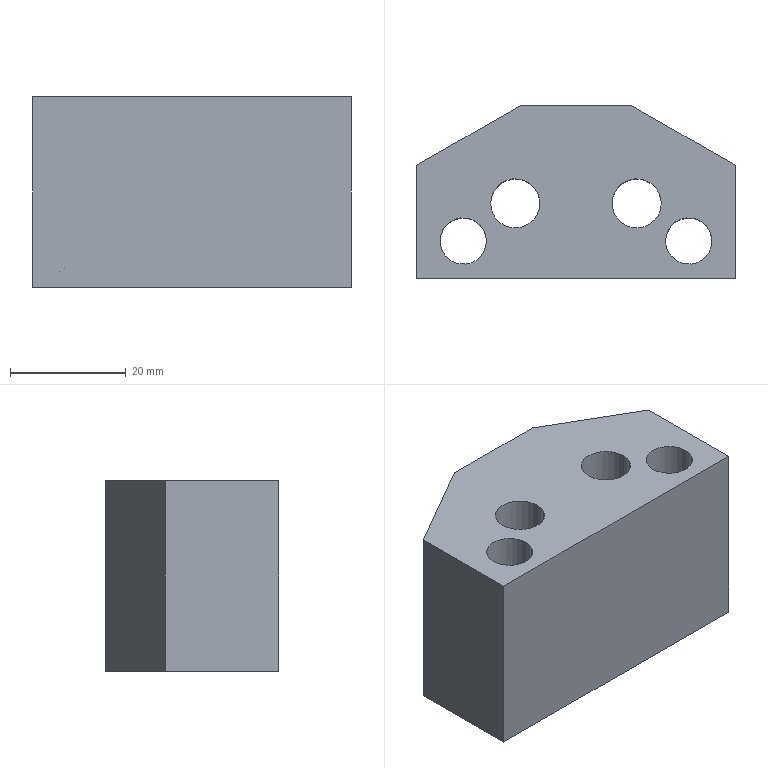Part | CATIA | 1 solid | 16 faces | box 55 x 30 x 33 mm | volume 41214 mm3 | plane 8 | cylinder 8 | commonest cylinder face diameters 8 x4 8.5 x4
STEP:
#1=CARTESIAN_POINT('',(27.5,-30.,38.));
#2=VERTEX_POINT('',#1);
#3=CARTESIAN_POINT('',(27.5,-30.,5.));
#4=VERTEX_POINT('',#3);
#5=CARTESIAN_POINT('',(27.5,-30.,21.5));
#6=DIRECTION('',(0.,0.,-1.));
#7=VECTOR('',#6,1.);
#8=LINE('',#5,#7);
#9=EDGE_CURVE('',#2,#4,#8,.T.);
#10=ORIENTED_EDGE('',*,*,#9,.F.);
#11=CARTESIAN_POINT('',(-27.5,-30.,38.));
#12=VERTEX_POINT('',#11);
#13=CARTESIAN_POINT('',(0.,-30.,38.));
#14=DIRECTION('',(-1.,0.,0.));
#15=VECTOR('',#14,1.);
#16=LINE('',#13,#15);
#17=EDGE_CURVE('',#2,#12,#16,.T.);
#18=ORIENTED_EDGE('',*,*,#17,.T.);
#19=CARTESIAN_POINT('',(-27.5,-30.,5.));
#20=VERTEX_POINT('',#19);
#21=CARTESIAN_POINT('',(-27.5,-30.,21.5));
#22=DIRECTION('',(0.,0.,-1.));
#23=VECTOR('',#22,1.);
#24=LINE('',#21,#23);
#25=EDGE_CURVE('',#12,#20,#24,.T.);
#26=ORIENTED_EDGE('',*,*,#25,.T.);
#27=CARTESIAN_POINT('',(0.,-30.,5.));
#28=DIRECTION('',(-1.,0.,0.));
#29=VECTOR('',#28,1.);
#30=LINE('',#27,#29);
#31=EDGE_CURVE('',#4,#20,#30,.T.);
#32=ORIENTED_EDGE('',*,*,#31,.F.);
#33=EDGE_LOOP('',(#10,#18,#26,#32));
#34=FACE_OUTER_BOUND('',#33,.T.);
#35=CARTESIAN_POINT('',(27.5,-30.,38.));
#36=DIRECTION('',(0.,-1.,0.));
#37=DIRECTION('',(-1.,0.,0.));
#38=AXIS2_PLACEMENT_3D('',#35,#36,#37);
#39=PLANE('',#38);
#40=ADVANCED_FACE('',(#34),#39,.T.);
#41=CARTESIAN_POINT('',(-27.5,-10.392,38.));
#42=VERTEX_POINT('',#41);
#43=CARTESIAN_POINT('',(-27.5,-10.392,5.));
#44=VERTEX_POINT('',#43);
#45=CARTESIAN_POINT('',(-27.5,-10.392,21.5));
#46=DIRECTION('',(0.,0.,-1.));
#47=VECTOR('',#46,1.);
#48=LINE('',#45,#47);
#49=EDGE_CURVE('',#42,#44,#48,.T.);
#50=ORIENTED_EDGE('',*,*,#49,.T.);
#51=CARTESIAN_POINT('',(-27.5,-20.196,5.));
#52=DIRECTION('',(0.,-1.,0.));
#53=VECTOR('',#52,1.);
#54=LINE('',#51,#53);
#55=EDGE_CURVE('',#20,#44,#54,.F.);
#56=ORIENTED_EDGE('',*,*,#55,.F.);
#57=ORIENTED_EDGE('',*,*,#25,.F.);
#58=CARTESIAN_POINT('',(-27.5,-20.196,38.));
#59=DIRECTION('',(0.,-1.,0.));
#60=VECTOR('',#59,1.);
#61=LINE('',#58,#60);
#62=EDGE_CURVE('',#12,#42,#61,.F.);
#63=ORIENTED_EDGE('',*,*,#62,.T.);
#64=EDGE_LOOP('',(#50,#56,#57,#63));
#65=FACE_OUTER_BOUND('',#64,.T.);
#66=CARTESIAN_POINT('',(-27.5,0.,38.));
#67=DIRECTION('',(1.,0.,0.));
#68=DIRECTION('',(0.,-1.,0.));
#69=AXIS2_PLACEMENT_3D('',#66,#67,#68);
#70=PLANE('',#69);
#71=ADVANCED_FACE('',(#65),#70,.F.);
#72=CARTESIAN_POINT('',(-9.5,0.,5.));
#73=VERTEX_POINT('',#72);
#74=CARTESIAN_POINT('',(-18.5,-5.196,5.));
#75=DIRECTION('',(-0.866,-0.5,0.));
#76=VECTOR('',#75,1.);
#77=LINE('',#74,#76);
#78=EDGE_CURVE('',#73,#44,#77,.T.);
#79=ORIENTED_EDGE('',*,*,#78,.T.);
#80=ORIENTED_EDGE('',*,*,#49,.F.);
#81=CARTESIAN_POINT('',(-9.5,0.,38.));
#82=VERTEX_POINT('',#81);
#83=CARTESIAN_POINT('',(-18.5,-5.196,38.));
#84=DIRECTION('',(-0.866,-0.5,0.));
#85=VECTOR('',#84,1.);
#86=LINE('',#83,#85);
#87=EDGE_CURVE('',#42,#82,#86,.F.);
#88=ORIENTED_EDGE('',*,*,#87,.T.);
#89=CARTESIAN_POINT('',(-9.5,0.,21.5));
#90=DIRECTION('',(0.,0.,-1.));
#91=VECTOR('',#90,1.);
#92=LINE('',#89,#91);
#93=EDGE_CURVE('',#82,#73,#92,.T.);
#94=ORIENTED_EDGE('',*,*,#93,.T.);
#95=EDGE_LOOP('',(#79,#80,#88,#94));
#96=FACE_OUTER_BOUND('',#95,.T.);
#97=CARTESIAN_POINT('',(-9.5,0.,44.6));
#98=DIRECTION('',(-0.5,0.866,0.));
#99=DIRECTION('',(0.,0.,-1.));
#100=AXIS2_PLACEMENT_3D('',#97,#98,#99);
#101=PLANE('',#100);
#102=ADVANCED_FACE('',(#96),#101,.T.);
#103=CARTESIAN_POINT('',(27.5,-10.392,38.));
#104=VERTEX_POINT('',#103);
#105=CARTESIAN_POINT('',(27.5,-10.392,5.));
#106=VERTEX_POINT('',#105);
#107=CARTESIAN_POINT('',(27.5,-10.392,21.5));
#108=DIRECTION('',(0.,0.,1.));
#109=VECTOR('',#108,1.);
#110=LINE('',#107,#109);
#111=EDGE_CURVE('',#104,#106,#110,.F.);
#112=ORIENTED_EDGE('',*,*,#111,.F.);
#113=CARTESIAN_POINT('',(27.5,-20.196,38.));
#114=DIRECTION('',(0.,1.,0.));
#115=VECTOR('',#114,1.);
#116=LINE('',#113,#115);
#117=EDGE_CURVE('',#104,#2,#116,.F.);
#118=ORIENTED_EDGE('',*,*,#117,.T.);
#119=ORIENTED_EDGE('',*,*,#9,.T.);
#120=CARTESIAN_POINT('',(27.5,-20.196,5.));
#121=DIRECTION('',(0.,1.,0.));
#122=VECTOR('',#121,1.);
#123=LINE('',#120,#122);
#124=EDGE_CURVE('',#106,#4,#123,.F.);
#125=ORIENTED_EDGE('',*,*,#124,.F.);
#126=EDGE_LOOP('',(#112,#118,#119,#125));
#127=FACE_OUTER_BOUND('',#126,.T.);
#128=CARTESIAN_POINT('',(27.5,-30.,38.));
#129=DIRECTION('',(-1.,0.,0.));
#130=DIRECTION('',(0.,1.,0.));
#131=AXIS2_PLACEMENT_3D('',#128,#129,#130);
#132=PLANE('',#131);
#133=ADVANCED_FACE('',(#127),#132,.F.);
#134=CARTESIAN_POINT('',(9.5,0.,5.));
#135=VERTEX_POINT('',#134);
#136=CARTESIAN_POINT('',(0.,0.,5.));
#137=DIRECTION('',(1.,0.,0.));
#138=VECTOR('',#137,1.);
#139=LINE('',#136,#138);
#140=EDGE_CURVE('',#73,#135,#139,.T.);
#141=ORIENTED_EDGE('',*,*,#140,.F.);
#142=ORIENTED_EDGE('',*,*,#93,.F.);
#143=CARTESIAN_POINT('',(9.5,0.,38.));
#144=VERTEX_POINT('',#143);
#145=CARTESIAN_POINT('',(0.,0.,38.));
#146=DIRECTION('',(1.,0.,0.));
#147=VECTOR('',#146,1.);
#148=LINE('',#145,#147);
#149=EDGE_CURVE('',#82,#144,#148,.T.);
#150=ORIENTED_EDGE('',*,*,#149,.T.);
#151=CARTESIAN_POINT('',(9.5,0.,21.5));
#152=DIRECTION('',(0.,0.,1.));
#153=VECTOR('',#152,1.);
#154=LINE('',#151,#153);
#155=EDGE_CURVE('',#144,#135,#154,.F.);
#156=ORIENTED_EDGE('',*,*,#155,.T.);
#157=EDGE_LOOP('',(#141,#142,#150,#156));
#158=FACE_OUTER_BOUND('',#157,.T.);
#159=CARTESIAN_POINT('',(-27.5,0.,38.));
#160=DIRECTION('',(0.,1.,0.));
#161=DIRECTION('',(1.,0.,0.));
#162=AXIS2_PLACEMENT_3D('',#159,#160,#161);
#163=PLANE('',#162);
#164=ADVANCED_FACE('',(#158),#163,.T.);
#165=CARTESIAN_POINT('',(18.5,-5.196,5.));
#166=DIRECTION('',(0.866,-0.5,0.));
#167=VECTOR('',#166,1.);
#168=LINE('',#165,#167);
#169=EDGE_CURVE('',#106,#135,#168,.F.);
#170=ORIENTED_EDGE('',*,*,#169,.T.);
#171=ORIENTED_EDGE('',*,*,#155,.F.);
#172=CARTESIAN_POINT('',(18.5,-5.196,38.));
#173=DIRECTION('',(0.866,-0.5,0.));
#174=VECTOR('',#173,1.);
#175=LINE('',#172,#174);
#176=EDGE_CURVE('',#144,#104,#175,.T.);
#177=ORIENTED_EDGE('',*,*,#176,.T.);
#178=ORIENTED_EDGE('',*,*,#111,.T.);
#179=EDGE_LOOP('',(#170,#171,#177,#178));
#180=FACE_OUTER_BOUND('',#179,.T.);
#181=CARTESIAN_POINT('',(9.5,0.,-1.6));
#182=DIRECTION('',(0.5,0.866,0.));
#183=DIRECTION('',(0.,0.,1.));
#184=AXIS2_PLACEMENT_3D('',#181,#182,#183);
#185=PLANE('',#184);
#186=ADVANCED_FACE('',(#180),#185,.T.);
#187=ORIENTED_EDGE('',*,*,#124,.T.);
#188=ORIENTED_EDGE('',*,*,#31,.T.);
#189=ORIENTED_EDGE('',*,*,#55,.T.);
#190=ORIENTED_EDGE('',*,*,#78,.F.);
#191=ORIENTED_EDGE('',*,*,#140,.T.);
#192=ORIENTED_EDGE('',*,*,#169,.F.);
#193=EDGE_LOOP('',(#187,#188,#189,#190,#191,#192));
#194=FACE_OUTER_BOUND('',#193,.T.);
#195=CARTESIAN_POINT('',(-14.23,-14.962,5.));
#196=VERTEX_POINT('',#195);
#197=CARTESIAN_POINT('',(-6.77,-19.038,5.));
#198=VERTEX_POINT('',#197);
#199=CARTESIAN_POINT('',(-10.5,-17.,5.));
#200=DIRECTION('',(0.,0.,-1.));
#201=AXIS2_PLACEMENT_3D('',#199,#200,$);
#202=CIRCLE('',#201,4.25);
#203=EDGE_CURVE('',#196,#198,#202,.T.);
#204=ORIENTED_EDGE('',*,*,#203,.F.);
#205=CARTESIAN_POINT('',(-10.5,-17.,5.));
#206=DIRECTION('',(0.,0.,-1.));
#207=AXIS2_PLACEMENT_3D('',#205,#206,$);
#208=CIRCLE('',#207,4.25);
#209=EDGE_CURVE('',#198,#196,#208,.T.);
#210=ORIENTED_EDGE('',*,*,#209,.F.);
#211=EDGE_LOOP('',(#204,#210));
#212=FACE_BOUND('',#211,.T.);
#213=CARTESIAN_POINT('',(6.77,-14.962,5.));
#214=VERTEX_POINT('',#213);
#215=CARTESIAN_POINT('',(14.23,-19.038,5.));
#216=VERTEX_POINT('',#215);
#217=CARTESIAN_POINT('',(10.5,-17.,5.));
#218=DIRECTION('',(0.,0.,-1.));
#219=AXIS2_PLACEMENT_3D('',#217,#218,$);
#220=CIRCLE('',#219,4.25);
#221=EDGE_CURVE('',#214,#216,#220,.T.);
#222=ORIENTED_EDGE('',*,*,#221,.F.);
#223=CARTESIAN_POINT('',(10.5,-17.,5.));
#224=DIRECTION('',(0.,0.,-1.));
#225=AXIS2_PLACEMENT_3D('',#223,#224,$);
#226=CIRCLE('',#225,4.25);
#227=EDGE_CURVE('',#216,#214,#226,.T.);
#228=ORIENTED_EDGE('',*,*,#227,.F.);
#229=EDGE_LOOP('',(#222,#228));
#230=FACE_BOUND('',#229,.T.);
#231=CARTESIAN_POINT('',(-23.01,-21.582,5.));
#232=VERTEX_POINT('',#231);
#233=CARTESIAN_POINT('',(-15.99,-25.418,5.));
#234=VERTEX_POINT('',#233);
#235=CARTESIAN_POINT('',(-19.5,-23.5,5.));
#236=DIRECTION('',(0.,0.,-1.));
#237=AXIS2_PLACEMENT_3D('',#235,#236,$);
#238=CIRCLE('',#237,4.);
#239=EDGE_CURVE('',#232,#234,#238,.T.);
#240=ORIENTED_EDGE('',*,*,#239,.F.);
#241=CARTESIAN_POINT('',(-19.5,-23.5,5.));
#242=DIRECTION('',(0.,0.,-1.));
#243=AXIS2_PLACEMENT_3D('',#241,#242,$);
#244=CIRCLE('',#243,4.);
#245=EDGE_CURVE('',#234,#232,#244,.T.);
#246=ORIENTED_EDGE('',*,*,#245,.F.);
#247=EDGE_LOOP('',(#240,#246));
#248=FACE_BOUND('',#247,.T.);
#249=CARTESIAN_POINT('',(15.99,-21.582,5.));
#250=VERTEX_POINT('',#249);
#251=CARTESIAN_POINT('',(23.01,-25.418,5.));
#252=VERTEX_POINT('',#251);
#253=CARTESIAN_POINT('',(19.5,-23.5,5.));
#254=DIRECTION('',(0.,0.,-1.));
#255=AXIS2_PLACEMENT_3D('',#253,#254,$);
#256=CIRCLE('',#255,4.);
#257=EDGE_CURVE('',#250,#252,#256,.T.);
#258=ORIENTED_EDGE('',*,*,#257,.F.);
#259=CARTESIAN_POINT('',(19.5,-23.5,5.));
#260=DIRECTION('',(0.,0.,-1.));
#261=AXIS2_PLACEMENT_3D('',#259,#260,$);
#262=CIRCLE('',#261,4.);
#263=EDGE_CURVE('',#252,#250,#262,.T.);
#264=ORIENTED_EDGE('',*,*,#263,.F.);
#265=EDGE_LOOP('',(#258,#264));
#266=FACE_BOUND('',#265,.T.);
#267=CARTESIAN_POINT('',(0.,0.,5.));
#268=DIRECTION('',(0.,0.,-1.));
#269=DIRECTION('',(1.,0.,0.));
#270=AXIS2_PLACEMENT_3D('',#267,#268,#269);
#271=PLANE('',#270);
#272=ADVANCED_FACE('',(#194,#212,#230,#248,#266),#271,.T.);
#273=ORIENTED_EDGE('',*,*,#176,.F.);
#274=ORIENTED_EDGE('',*,*,#149,.F.);
#275=ORIENTED_EDGE('',*,*,#87,.F.);
#276=ORIENTED_EDGE('',*,*,#62,.F.);
#277=ORIENTED_EDGE('',*,*,#17,.F.);
#278=ORIENTED_EDGE('',*,*,#117,.F.);
#279=EDGE_LOOP('',(#273,#274,#275,#276,#277,#278));
#280=FACE_OUTER_BOUND('',#279,.T.);
#281=CARTESIAN_POINT('',(-14.23,-14.962,38.));
#282=VERTEX_POINT('',#281);
#283=CARTESIAN_POINT('',(-6.77,-19.038,38.));
#284=VERTEX_POINT('',#283);
#285=CARTESIAN_POINT('',(-10.5,-17.,38.));
#286=DIRECTION('',(0.,0.,-1.));
#287=AXIS2_PLACEMENT_3D('',#285,#286,$);
#288=CIRCLE('',#287,4.25);
#289=EDGE_CURVE('',#282,#284,#288,.T.);
#290=ORIENTED_EDGE('',*,*,#289,.T.);
#291=CARTESIAN_POINT('',(-10.5,-17.,38.));
#292=DIRECTION('',(0.,0.,-1.));
#293=AXIS2_PLACEMENT_3D('',#291,#292,$);
#294=CIRCLE('',#293,4.25);
#295=EDGE_CURVE('',#284,#282,#294,.T.);
#296=ORIENTED_EDGE('',*,*,#295,.T.);
#297=EDGE_LOOP('',(#290,#296));
#298=FACE_BOUND('',#297,.T.);
#299=CARTESIAN_POINT('',(6.77,-14.962,38.));
#300=VERTEX_POINT('',#299);
#301=CARTESIAN_POINT('',(14.23,-19.038,38.));
#302=VERTEX_POINT('',#301);
#303=CARTESIAN_POINT('',(10.5,-17.,38.));
#304=DIRECTION('',(0.,0.,-1.));
#305=AXIS2_PLACEMENT_3D('',#303,#304,$);
#306=CIRCLE('',#305,4.25);
#307=EDGE_CURVE('',#300,#302,#306,.T.);
#308=ORIENTED_EDGE('',*,*,#307,.T.);
#309=CARTESIAN_POINT('',(10.5,-17.,38.));
#310=DIRECTION('',(0.,0.,-1.));
#311=AXIS2_PLACEMENT_3D('',#309,#310,$);
#312=CIRCLE('',#311,4.25);
#313=EDGE_CURVE('',#302,#300,#312,.T.);
#314=ORIENTED_EDGE('',*,*,#313,.T.);
#315=EDGE_LOOP('',(#308,#314));
#316=FACE_BOUND('',#315,.T.);
#317=CARTESIAN_POINT('',(-23.01,-21.582,38.));
#318=VERTEX_POINT('',#317);
#319=CARTESIAN_POINT('',(-15.99,-25.418,38.));
#320=VERTEX_POINT('',#319);
#321=CARTESIAN_POINT('',(-19.5,-23.5,38.));
#322=DIRECTION('',(0.,0.,-1.));
#323=AXIS2_PLACEMENT_3D('',#321,#322,$);
#324=CIRCLE('',#323,4.);
#325=EDGE_CURVE('',#318,#320,#324,.T.);
#326=ORIENTED_EDGE('',*,*,#325,.T.);
#327=CARTESIAN_POINT('',(-19.5,-23.5,38.));
#328=DIRECTION('',(0.,0.,-1.));
#329=AXIS2_PLACEMENT_3D('',#327,#328,$);
#330=CIRCLE('',#329,4.);
#331=EDGE_CURVE('',#320,#318,#330,.T.);
#332=ORIENTED_EDGE('',*,*,#331,.T.);
#333=EDGE_LOOP('',(#326,#332));
#334=FACE_BOUND('',#333,.T.);
#335=CARTESIAN_POINT('',(15.99,-21.582,38.));
#336=VERTEX_POINT('',#335);
#337=CARTESIAN_POINT('',(23.01,-25.418,38.));
#338=VERTEX_POINT('',#337);
#339=CARTESIAN_POINT('',(19.5,-23.5,38.));
#340=DIRECTION('',(0.,0.,-1.));
#341=AXIS2_PLACEMENT_3D('',#339,#340,$);
#342=CIRCLE('',#341,4.);
#343=EDGE_CURVE('',#336,#338,#342,.T.);
#344=ORIENTED_EDGE('',*,*,#343,.T.);
#345=CARTESIAN_POINT('',(19.5,-23.5,38.));
#346=DIRECTION('',(0.,0.,-1.));
#347=AXIS2_PLACEMENT_3D('',#345,#346,$);
#348=CIRCLE('',#347,4.);
#349=EDGE_CURVE('',#338,#336,#348,.T.);
#350=ORIENTED_EDGE('',*,*,#349,.T.);
#351=EDGE_LOOP('',(#344,#350));
#352=FACE_BOUND('',#351,.T.);
#353=CARTESIAN_POINT('',(0.,0.,38.));
#354=DIRECTION('',(0.,0.,-1.));
#355=DIRECTION('',(1.,0.,0.));
#356=AXIS2_PLACEMENT_3D('',#353,#354,#355);
#357=PLANE('',#356);
#358=ADVANCED_FACE('',(#280,#298,#316,#334,#352),#357,.F.);
#359=ORIENTED_EDGE('',*,*,#331,.F.);
#360=CARTESIAN_POINT('',(-15.99,-25.418,21.5));
#361=DIRECTION('',(0.,0.,-1.));
#362=VECTOR('',#361,1.);
#363=LINE('',#360,#362);
#364=EDGE_CURVE('',#234,#320,#363,.F.);
#365=ORIENTED_EDGE('',*,*,#364,.F.);
#366=ORIENTED_EDGE('',*,*,#245,.T.);
#367=CARTESIAN_POINT('',(-23.01,-21.582,21.5));
#368=DIRECTION('',(0.,0.,-1.));
#369=VECTOR('',#368,1.);
#370=LINE('',#367,#369);
#371=EDGE_CURVE('',#232,#318,#370,.F.);
#372=ORIENTED_EDGE('',*,*,#371,.T.);
#373=EDGE_LOOP('',(#359,#365,#366,#372));
#374=FACE_OUTER_BOUND('',#373,.T.);
#375=CARTESIAN_POINT('',(-19.5,-23.5,37.9));
#376=DIRECTION('',(0.,0.,-1.));
#377=DIRECTION('',(0.8776,-0.4794,0.));
#378=AXIS2_PLACEMENT_3D('',#375,#376,#377);
#379=CYLINDRICAL_SURFACE('',#378,4.);
#380=ADVANCED_FACE('',(#374),#379,.F.);
#381=ORIENTED_EDGE('',*,*,#325,.F.);
#382=ORIENTED_EDGE('',*,*,#371,.F.);
#383=ORIENTED_EDGE('',*,*,#239,.T.);
#384=ORIENTED_EDGE('',*,*,#364,.T.);
#385=EDGE_LOOP('',(#381,#382,#383,#384));
#386=FACE_OUTER_BOUND('',#385,.T.);
#387=ADVANCED_FACE('',(#386),#379,.F.);
#388=ORIENTED_EDGE('',*,*,#313,.F.);
#389=CARTESIAN_POINT('',(14.23,-19.038,21.5));
#390=DIRECTION('',(0.,0.,-1.));
#391=VECTOR('',#390,1.);
#392=LINE('',#389,#391);
#393=EDGE_CURVE('',#216,#302,#392,.F.);
#394=ORIENTED_EDGE('',*,*,#393,.F.);
#395=ORIENTED_EDGE('',*,*,#227,.T.);
#396=CARTESIAN_POINT('',(6.77,-14.962,21.5));
#397=DIRECTION('',(0.,0.,-1.));
#398=VECTOR('',#397,1.);
#399=LINE('',#396,#398);
#400=EDGE_CURVE('',#214,#300,#399,.F.);
#401=ORIENTED_EDGE('',*,*,#400,.T.);
#402=EDGE_LOOP('',(#388,#394,#395,#401));
#403=FACE_OUTER_BOUND('',#402,.T.);
#404=CARTESIAN_POINT('',(10.5,-17.,37.9));
#405=DIRECTION('',(0.,0.,-1.));
#406=DIRECTION('',(0.8776,-0.4794,0.));
#407=AXIS2_PLACEMENT_3D('',#404,#405,#406);
#408=CYLINDRICAL_SURFACE('',#407,4.25);
#409=ADVANCED_FACE('',(#403),#408,.F.);
#410=ORIENTED_EDGE('',*,*,#307,.F.);
#411=ORIENTED_EDGE('',*,*,#400,.F.);
#412=ORIENTED_EDGE('',*,*,#221,.T.);
#413=ORIENTED_EDGE('',*,*,#393,.T.);
#414=EDGE_LOOP('',(#410,#411,#412,#413));
#415=FACE_OUTER_BOUND('',#414,.T.);
#416=ADVANCED_FACE('',(#415),#408,.F.);
#417=ORIENTED_EDGE('',*,*,#349,.F.);
#418=CARTESIAN_POINT('',(23.01,-25.418,21.5));
#419=DIRECTION('',(0.,0.,-1.));
#420=VECTOR('',#419,1.);
#421=LINE('',#418,#420);
#422=EDGE_CURVE('',#252,#338,#421,.F.);
#423=ORIENTED_EDGE('',*,*,#422,.F.);
#424=ORIENTED_EDGE('',*,*,#263,.T.);
#425=CARTESIAN_POINT('',(15.99,-21.582,21.5));
#426=DIRECTION('',(0.,0.,-1.));
#427=VECTOR('',#426,1.);
#428=LINE('',#425,#427);
#429=EDGE_CURVE('',#250,#336,#428,.F.);
#430=ORIENTED_EDGE('',*,*,#429,.T.);
#431=EDGE_LOOP('',(#417,#423,#424,#430));
#432=FACE_OUTER_BOUND('',#431,.T.);
#433=CARTESIAN_POINT('',(19.5,-23.5,37.9));
#434=DIRECTION('',(0.,0.,-1.));
#435=DIRECTION('',(0.8776,-0.4794,0.));
#436=AXIS2_PLACEMENT_3D('',#433,#434,#435);
#437=CYLINDRICAL_SURFACE('',#436,4.);
#438=ADVANCED_FACE('',(#432),#437,.F.);
#439=ORIENTED_EDGE('',*,*,#343,.F.);
#440=ORIENTED_EDGE('',*,*,#429,.F.);
#441=ORIENTED_EDGE('',*,*,#257,.T.);
#442=ORIENTED_EDGE('',*,*,#422,.T.);
#443=EDGE_LOOP('',(#439,#440,#441,#442));
#444=FACE_OUTER_BOUND('',#443,.T.);
#445=ADVANCED_FACE('',(#444),#437,.F.);
#446=ORIENTED_EDGE('',*,*,#295,.F.);
#447=CARTESIAN_POINT('',(-6.77,-19.038,21.5));
#448=DIRECTION('',(0.,0.,-1.));
#449=VECTOR('',#448,1.);
#450=LINE('',#447,#449);
#451=EDGE_CURVE('',#198,#284,#450,.F.);
#452=ORIENTED_EDGE('',*,*,#451,.F.);
#453=ORIENTED_EDGE('',*,*,#209,.T.);
#454=CARTESIAN_POINT('',(-14.23,-14.962,21.5));
#455=DIRECTION('',(0.,0.,-1.));
#456=VECTOR('',#455,1.);
#457=LINE('',#454,#456);
#458=EDGE_CURVE('',#196,#282,#457,.F.);
#459=ORIENTED_EDGE('',*,*,#458,.T.);
#460=EDGE_LOOP('',(#446,#452,#453,#459));
#461=FACE_OUTER_BOUND('',#460,.T.);
#462=CARTESIAN_POINT('',(-10.5,-17.,37.9));
#463=DIRECTION('',(0.,0.,-1.));
#464=DIRECTION('',(0.8776,-0.4794,0.));
#465=AXIS2_PLACEMENT_3D('',#462,#463,#464);
#466=CYLINDRICAL_SURFACE('',#465,4.25);
#467=ADVANCED_FACE('',(#461),#466,.F.);
#468=ORIENTED_EDGE('',*,*,#289,.F.);
#469=ORIENTED_EDGE('',*,*,#458,.F.);
#470=ORIENTED_EDGE('',*,*,#203,.T.);
#471=ORIENTED_EDGE('',*,*,#451,.T.);
#472=EDGE_LOOP('',(#468,#469,#470,#471));
#473=FACE_OUTER_BOUND('',#472,.T.);
#474=ADVANCED_FACE('',(#473),#466,.F.);
#475=CLOSED_SHELL('',(#40,#71,#102,#133,#164,#186,#272,#358,#380,#387,#409,#416,#438,#445,#467,#474));
#476=MANIFOLD_SOLID_BREP('',#475);
#477=(LENGTH_UNIT()NAMED_UNIT(*)SI_UNIT(.MILLI.,.METRE.));
#478=UNCERTAINTY_MEASURE_WITH_UNIT(LENGTH_MEASURE(0.005),#477,'','');
#479=(NAMED_UNIT(*)PLANE_ANGLE_UNIT()SI_UNIT($,.RADIAN.));
#480=(NAMED_UNIT(*)SI_UNIT($,.STERADIAN.)SOLID_ANGLE_UNIT());
#481=(GEOMETRIC_REPRESENTATION_CONTEXT(3)GLOBAL_UNCERTAINTY_ASSIGNED_CONTEXT((#478))GLOBAL_UNIT_ASSIGNED_CONTEXT((#477,#479,#480))REPRESENTATION_CONTEXT('',''));
#482=ADVANCED_BREP_SHAPE_REPRESENTATION('',(#476),#481);